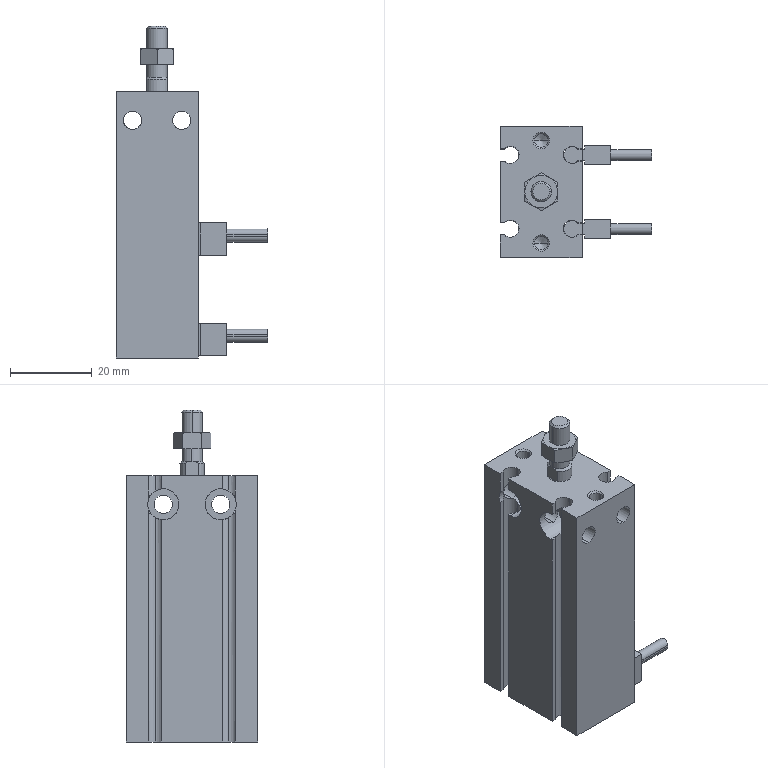Part | SolidWorks | 5 solids | 219 faces | box 37 x 32 x 81 mm | volume 32994 mm3 | cylinder 90 | plane 85 | cone 44 | commonest cylinder face diameters 7.6 x20 4.5 x16 3.242 x8 4.2 x8 2.1 x6 2.7 x6